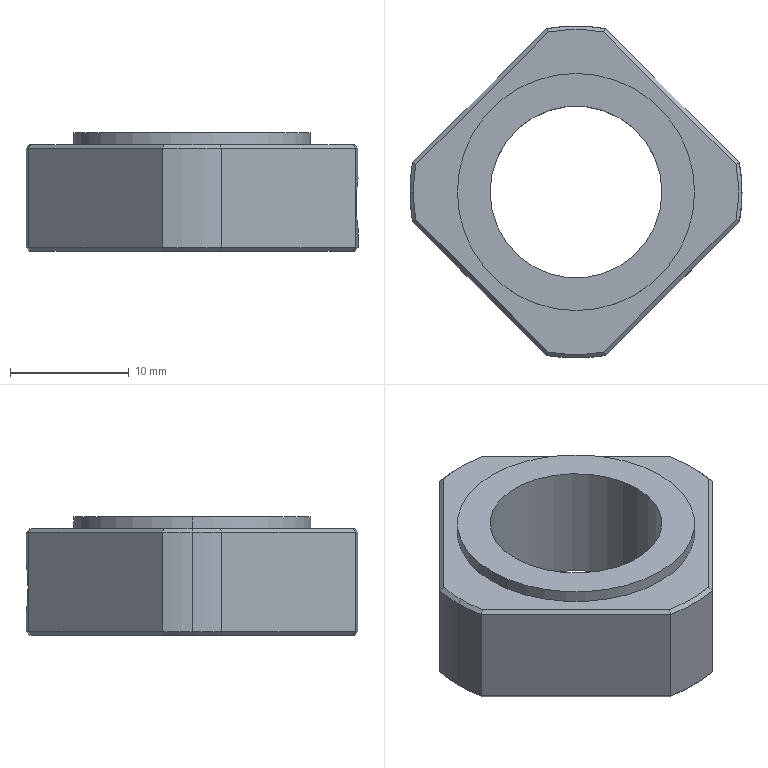Part | STEP file | Square precision nut RN_M16×1.5P | 1 solid | 54 faces | box 28 x 28 x 10 mm | volume 3186 mm3 | plane 31 | cylinder 13 | cone 10 | commonest cylinder face diameters 28 x5 4.2 x4 14.5 x2 20 x2